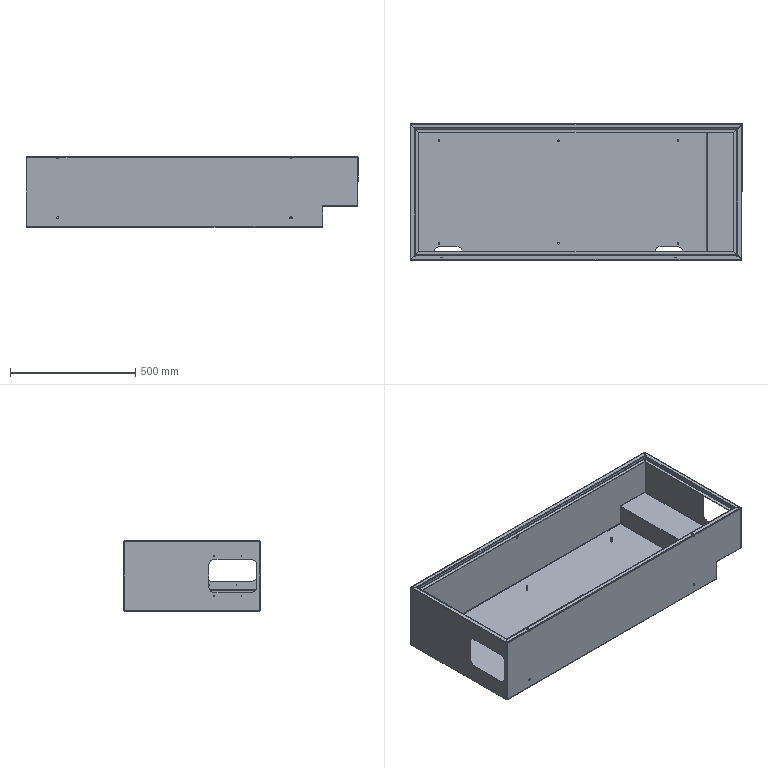Part | SolidWorks | features BaseBody 3 | 3 solids | 268 faces | box 1324 x 545 x 280 mm | volume 3651859 mm3 | plane 140 | cylinder 106 | spline 20 | cone 2 | commonest cylinder face diameters 6 x32 2 x24 3.3 x16 40 x14 9 x10 4 x4